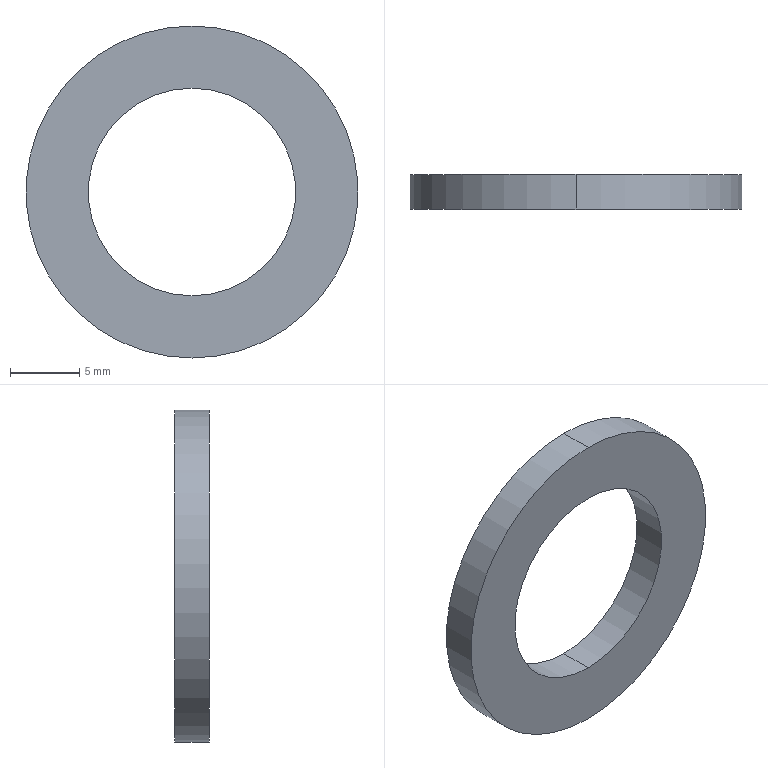Part | SolidWorks | features Revolution 1 | 1 solid | 6 faces | box 24 x 2.5 x 24 mm | volume 689.187 mm3 | cylinder 4 | plane 2 | commonest cylinder face diameters 15 x2 24 x2
STEP:
#1=CARTESIAN_POINT('',(0.,11.145,-12.));
#2=VERTEX_POINT('',#1);
#3=CARTESIAN_POINT('',(0.,11.145,12.));
#4=VERTEX_POINT('',#3);
#5=CARTESIAN_POINT('',(0.,11.145,0.));
#6=DIRECTION('',(0.,-1.,0.));
#7=DIRECTION('',(0.,0.,-1.));
#8=AXIS2_PLACEMENT_3D('',#5,#6,#7);
#9=CIRCLE('',#8,12.);
#10=EDGE_CURVE('',#2,#4,#9,.T.);
#11=ORIENTED_EDGE('',*,*,#10,.T.);
#12=CARTESIAN_POINT('',(0.,8.645,12.));
#13=VERTEX_POINT('',#12);
#14=CARTESIAN_POINT('',(0.,0.,12.));
#15=DIRECTION('',(0.,-1.,0.));
#16=VECTOR('',#15,1000.);
#17=LINE('',#14,#16);
#18=EDGE_CURVE('',#4,#13,#17,.T.);
#19=ORIENTED_EDGE('',*,*,#18,.T.);
#20=CARTESIAN_POINT('',(0.,8.645,-12.));
#21=VERTEX_POINT('',#20);
#22=CARTESIAN_POINT('',(0.,8.645,0.));
#23=DIRECTION('',(0.,-1.,0.));
#24=DIRECTION('',(0.,0.,-1.));
#25=AXIS2_PLACEMENT_3D('',#22,#23,#24);
#26=CIRCLE('',#25,12.);
#27=EDGE_CURVE('',#21,#13,#26,.T.);
#28=ORIENTED_EDGE('',*,*,#27,.F.);
#29=CARTESIAN_POINT('',(0.,0.,-12.));
#30=DIRECTION('',(0.,-1.,0.));
#31=VECTOR('',#30,1000.);
#32=LINE('',#29,#31);
#33=EDGE_CURVE('',#2,#21,#32,.T.);
#34=ORIENTED_EDGE('',*,*,#33,.F.);
#35=EDGE_LOOP('',(#11,#19,#28,#34));
#36=FACE_OUTER_BOUND('',#35,.T.);
#37=CARTESIAN_POINT('',(0.,0.,0.));
#38=DIRECTION('',(0.,-1.,0.));
#39=DIRECTION('',(0.,0.,-1.));
#40=AXIS2_PLACEMENT_3D('',#37,#38,#39);
#41=CYLINDRICAL_SURFACE('',#40,12.);
#42=ADVANCED_FACE('',(#36),#41,.T.);
#43=CARTESIAN_POINT('',(0.,11.145,7.5));
#44=VERTEX_POINT('',#43);
#45=CARTESIAN_POINT('',(0.,11.145,-7.5));
#46=VERTEX_POINT('',#45);
#47=CARTESIAN_POINT('',(0.,11.145,0.));
#48=DIRECTION('',(0.,-1.,0.));
#49=DIRECTION('',(0.,0.,-1.));
#50=AXIS2_PLACEMENT_3D('',#47,#48,#49);
#51=CIRCLE('',#50,7.5);
#52=EDGE_CURVE('',#44,#46,#51,.T.);
#53=ORIENTED_EDGE('',*,*,#52,.F.);
#54=CARTESIAN_POINT('',(0.,8.645,7.5));
#55=VERTEX_POINT('',#54);
#56=CARTESIAN_POINT('',(0.,0.,7.5));
#57=DIRECTION('',(0.,-1.,0.));
#58=VECTOR('',#57,1000.);
#59=LINE('',#56,#58);
#60=EDGE_CURVE('',#44,#55,#59,.T.);
#61=ORIENTED_EDGE('',*,*,#60,.T.);
#62=CARTESIAN_POINT('',(0.,8.645,-7.5));
#63=VERTEX_POINT('',#62);
#64=CARTESIAN_POINT('',(0.,8.645,0.));
#65=DIRECTION('',(0.,-1.,0.));
#66=DIRECTION('',(0.,0.,-1.));
#67=AXIS2_PLACEMENT_3D('',#64,#65,#66);
#68=CIRCLE('',#67,7.5);
#69=EDGE_CURVE('',#55,#63,#68,.T.);
#70=ORIENTED_EDGE('',*,*,#69,.T.);
#71=CARTESIAN_POINT('',(0.,0.,-7.5));
#72=DIRECTION('',(0.,-1.,0.));
#73=VECTOR('',#72,1000.);
#74=LINE('',#71,#73);
#75=EDGE_CURVE('',#46,#63,#74,.T.);
#76=ORIENTED_EDGE('',*,*,#75,.F.);
#77=EDGE_LOOP('',(#53,#61,#70,#76));
#78=FACE_OUTER_BOUND('',#77,.T.);
#79=CARTESIAN_POINT('',(0.,0.,0.));
#80=DIRECTION('',(0.,-1.,0.));
#81=DIRECTION('',(0.,0.,-1.));
#82=AXIS2_PLACEMENT_3D('',#79,#80,#81);
#83=CYLINDRICAL_SURFACE('',#82,7.5);
#84=ADVANCED_FACE('',(#78),#83,.F.);
#85=ORIENTED_EDGE('',*,*,#60,.F.);
#86=CARTESIAN_POINT('',(0.,11.145,0.));
#87=DIRECTION('',(0.,-1.,0.));
#88=DIRECTION('',(0.,0.,-1.));
#89=AXIS2_PLACEMENT_3D('',#86,#87,#88);
#90=CIRCLE('',#89,7.5);
#91=EDGE_CURVE('',#46,#44,#90,.T.);
#92=ORIENTED_EDGE('',*,*,#91,.F.);
#93=ORIENTED_EDGE('',*,*,#75,.T.);
#94=CARTESIAN_POINT('',(0.,8.645,0.));
#95=DIRECTION('',(0.,-1.,0.));
#96=DIRECTION('',(0.,0.,-1.));
#97=AXIS2_PLACEMENT_3D('',#94,#95,#96);
#98=CIRCLE('',#97,7.5);
#99=EDGE_CURVE('',#63,#55,#98,.T.);
#100=ORIENTED_EDGE('',*,*,#99,.T.);
#101=EDGE_LOOP('',(#85,#92,#93,#100));
#102=FACE_OUTER_BOUND('',#101,.T.);
#103=CARTESIAN_POINT('',(0.,0.,0.));
#104=DIRECTION('',(0.,-1.,0.));
#105=DIRECTION('',(0.,0.,-1.));
#106=AXIS2_PLACEMENT_3D('',#103,#104,#105);
#107=CYLINDRICAL_SURFACE('',#106,7.5);
#108=ADVANCED_FACE('',(#102),#107,.F.);
#109=ORIENTED_EDGE('',*,*,#10,.F.);
#110=CARTESIAN_POINT('',(0.,11.145,0.));
#111=DIRECTION('',(0.,-1.,0.));
#112=DIRECTION('',(0.,0.,-1.));
#113=AXIS2_PLACEMENT_3D('',#110,#111,#112);
#114=CIRCLE('',#113,12.);
#115=EDGE_CURVE('',#4,#2,#114,.T.);
#116=ORIENTED_EDGE('',*,*,#115,.F.);
#117=EDGE_LOOP('',(#109,#116));
#118=FACE_OUTER_BOUND('',#117,.T.);
#119=ORIENTED_EDGE('',*,*,#91,.T.);
#120=ORIENTED_EDGE('',*,*,#52,.T.);
#121=EDGE_LOOP('',(#119,#120));
#122=FACE_BOUND('',#121,.T.);
#123=CARTESIAN_POINT('',(-7.5,11.145,0.));
#124=DIRECTION('',(0.,-1.,0.));
#125=DIRECTION('',(0.,0.,-1.));
#126=AXIS2_PLACEMENT_3D('',#123,#124,#125);
#127=PLANE('',#126);
#128=ADVANCED_FACE('',(#118,#122),#127,.F.);
#129=ORIENTED_EDGE('',*,*,#18,.F.);
#130=ORIENTED_EDGE('',*,*,#115,.T.);
#131=ORIENTED_EDGE('',*,*,#33,.T.);
#132=CARTESIAN_POINT('',(0.,8.645,0.));
#133=DIRECTION('',(0.,-1.,0.));
#134=DIRECTION('',(0.,0.,-1.));
#135=AXIS2_PLACEMENT_3D('',#132,#133,#134);
#136=CIRCLE('',#135,12.);
#137=EDGE_CURVE('',#13,#21,#136,.T.);
#138=ORIENTED_EDGE('',*,*,#137,.F.);
#139=EDGE_LOOP('',(#129,#130,#131,#138));
#140=FACE_OUTER_BOUND('',#139,.T.);
#141=CARTESIAN_POINT('',(0.,0.,0.));
#142=DIRECTION('',(0.,-1.,0.));
#143=DIRECTION('',(0.,0.,-1.));
#144=AXIS2_PLACEMENT_3D('',#141,#142,#143);
#145=CYLINDRICAL_SURFACE('',#144,12.);
#146=ADVANCED_FACE('',(#140),#145,.T.);
#147=ORIENTED_EDGE('',*,*,#99,.F.);
#148=ORIENTED_EDGE('',*,*,#69,.F.);
#149=EDGE_LOOP('',(#147,#148));
#150=FACE_BOUND('',#149,.T.);
#151=ORIENTED_EDGE('',*,*,#27,.T.);
#152=ORIENTED_EDGE('',*,*,#137,.T.);
#153=EDGE_LOOP('',(#151,#152));
#154=FACE_OUTER_BOUND('',#153,.T.);
#155=CARTESIAN_POINT('',(-7.5,8.645,0.));
#156=DIRECTION('',(0.,1.,0.));
#157=DIRECTION('',(0.,0.,1.));
#158=AXIS2_PLACEMENT_3D('',#155,#156,#157);
#159=PLANE('',#158);
#160=ADVANCED_FACE('',(#150,#154),#159,.F.);
#161=CLOSED_SHELL('',(#42,#84,#108,#128,#146,#160));
#162=MANIFOLD_SOLID_BREP('',#161);
#163=CARTESIAN_POINT('',(0.,0.,0.));
#164=DIRECTION('',(0.,0.,1.));
#165=DIRECTION('',(1.,0.,0.));
#166=AXIS2_PLACEMENT_3D('',#163,#164,#165);
#167=(LENGTH_UNIT()NAMED_UNIT(*)SI_UNIT(.MILLI.,.METRE.));
#168=UNCERTAINTY_MEASURE_WITH_UNIT(LENGTH_MEASURE(0.00001),#167,'','');
#169=(NAMED_UNIT(*)PLANE_ANGLE_UNIT()SI_UNIT($,.RADIAN.));
#170=(NAMED_UNIT(*)SI_UNIT($,.STERADIAN.)SOLID_ANGLE_UNIT());
#171=(GEOMETRIC_REPRESENTATION_CONTEXT(3)GLOBAL_UNCERTAINTY_ASSIGNED_CONTEXT((#168))GLOBAL_UNIT_ASSIGNED_CONTEXT((#167,#169,#170))REPRESENTATION_CONTEXT('',''));
#172=ADVANCED_BREP_SHAPE_REPRESENTATION('',(#162,#166),#171);